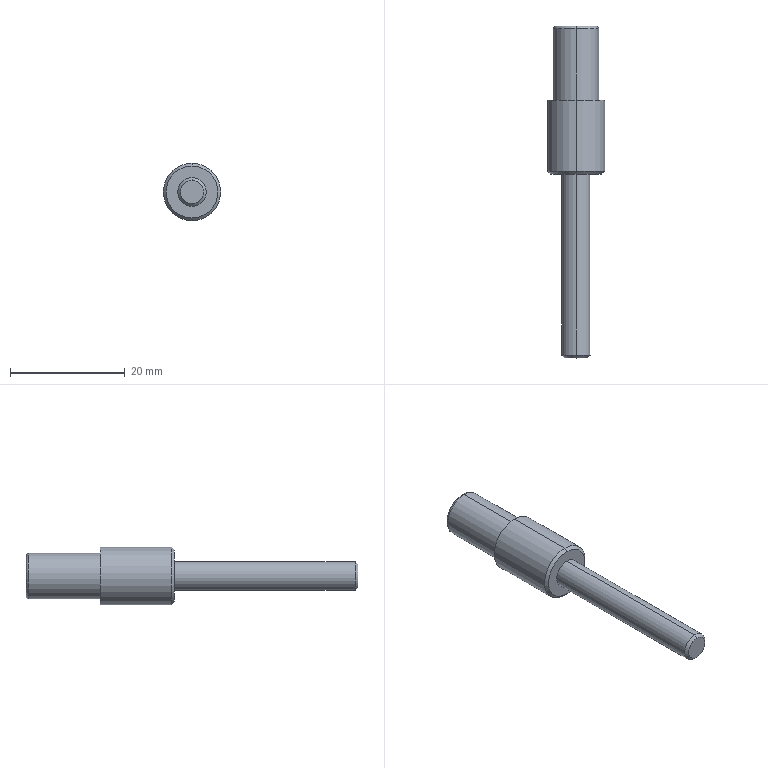Part | SolidWorks | features RefAxis 3, 3DProfileFeature 1, ICE 1, RevCut 1, Revolution 1 | 1 solid | 30 faces | box 10 x 57.8 x 10 mm | volume 2265 mm3 | plane 16 | cone 6 | cylinder 6 | torus 2 | commonest cylinder face diameters 5 x2 8 x2 10 x2
STEP:
#1=CARTESIAN_POINT('',(0.,22.934,0.));
#2=VERTEX_POINT('',#1);
#3=CARTESIAN_POINT('',(0.,23.8,1.5));
#4=VERTEX_POINT('',#3);
#5=CARTESIAN_POINT('',(0.,22.934,0.));
#6=DIRECTION('',(0.,0.5,0.866));
#7=VECTOR('',#6,1000.);
#8=LINE('',#5,#7);
#9=EDGE_CURVE('',#2,#4,#8,.T.);
#10=ORIENTED_EDGE('',*,*,#9,.F.);
#11=CARTESIAN_POINT('',(0.,23.8,-1.5));
#12=VERTEX_POINT('',#11);
#13=CARTESIAN_POINT('',(0.,22.934,0.));
#14=DIRECTION('',(0.,0.5,-0.866));
#15=VECTOR('',#14,1000.);
#16=LINE('',#13,#15);
#17=EDGE_CURVE('',#2,#12,#16,.T.);
#18=ORIENTED_EDGE('',*,*,#17,.T.);
#19=CARTESIAN_POINT('',(-0.75,23.8,-1.299));
#20=VERTEX_POINT('',#19);
#21=CARTESIAN_POINT('',(0.,23.8,0.));
#22=DIRECTION('',(0.,-1.,0.));
#23=DIRECTION('',(0.,0.,1.));
#24=AXIS2_PLACEMENT_3D('',#21,#22,#23);
#25=CIRCLE('',#24,1.5);
#26=EDGE_CURVE('',#20,#12,#25,.T.);
#27=ORIENTED_EDGE('',*,*,#26,.F.);
#28=CARTESIAN_POINT('',(-1.5,23.8,0.));
#29=VERTEX_POINT('',#28);
#30=CARTESIAN_POINT('',(0.,23.8,0.));
#31=DIRECTION('',(0.,-1.,0.));
#32=DIRECTION('',(0.,0.,1.));
#33=AXIS2_PLACEMENT_3D('',#30,#31,#32);
#34=CIRCLE('',#33,1.5);
#35=EDGE_CURVE('',#29,#20,#34,.T.);
#36=ORIENTED_EDGE('',*,*,#35,.F.);
#37=CARTESIAN_POINT('',(-0.75,23.8,1.299));
#38=VERTEX_POINT('',#37);
#39=CARTESIAN_POINT('',(0.,23.8,0.));
#40=DIRECTION('',(0.,-1.,0.));
#41=DIRECTION('',(0.,0.,1.));
#42=AXIS2_PLACEMENT_3D('',#39,#40,#41);
#43=CIRCLE('',#42,1.5);
#44=EDGE_CURVE('',#38,#29,#43,.T.);
#45=ORIENTED_EDGE('',*,*,#44,.F.);
#46=CARTESIAN_POINT('',(0.,23.8,0.));
#47=DIRECTION('',(0.,-1.,0.));
#48=DIRECTION('',(0.,0.,1.));
#49=AXIS2_PLACEMENT_3D('',#46,#47,#48);
#50=CIRCLE('',#49,1.5);
#51=EDGE_CURVE('',#4,#38,#50,.T.);
#52=ORIENTED_EDGE('',*,*,#51,.F.);
#53=EDGE_LOOP('',(#10,#18,#27,#36,#45,#52));
#54=FACE_OUTER_BOUND('',#53,.T.);
#55=CARTESIAN_POINT('',(0.,1022.934,0.));
#56=DIRECTION('',(0.,1.,0.));
#57=DIRECTION('',(0.,0.,1.));
#58=AXIS2_PLACEMENT_3D('',#55,#56,#57);
#59=CONICAL_SURFACE('',#58,1732.051,1.047);
#60=ADVANCED_FACE('',(#54),#59,.F.);
#61=CARTESIAN_POINT('',(0.,-32.,2.01));
#62=VERTEX_POINT('',#61);
#63=CARTESIAN_POINT('',(0.,-32.,-2.01));
#64=VERTEX_POINT('',#63);
#65=CARTESIAN_POINT('',(0.,-32.,0.));
#66=DIRECTION('',(0.,1.,0.));
#67=DIRECTION('',(0.,0.,1.));
#68=AXIS2_PLACEMENT_3D('',#65,#66,#67);
#69=CIRCLE('',#68,2.01);
#70=EDGE_CURVE('',#62,#64,#69,.T.);
#71=ORIENTED_EDGE('',*,*,#70,.T.);
#72=CARTESIAN_POINT('',(0.,-31.51,-2.5));
#73=VERTEX_POINT('',#72);
#74=CARTESIAN_POINT('',(0.,-32.,-2.01));
#75=DIRECTION('',(0.,0.7071,-0.7071));
#76=VECTOR('',#75,1000.);
#77=LINE('',#74,#76);
#78=EDGE_CURVE('',#64,#73,#77,.T.);
#79=ORIENTED_EDGE('',*,*,#78,.T.);
#80=CARTESIAN_POINT('',(0.,-31.51,2.5));
#81=VERTEX_POINT('',#80);
#82=CARTESIAN_POINT('',(0.,-31.51,0.));
#83=DIRECTION('',(0.,1.,0.));
#84=DIRECTION('',(0.,0.,1.));
#85=AXIS2_PLACEMENT_3D('',#82,#83,#84);
#86=CIRCLE('',#85,2.5);
#87=EDGE_CURVE('',#81,#73,#86,.T.);
#88=ORIENTED_EDGE('',*,*,#87,.F.);
#89=CARTESIAN_POINT('',(0.,-32.,2.01));
#90=DIRECTION('',(0.,0.7071,0.7071));
#91=VECTOR('',#90,1000.);
#92=LINE('',#89,#91);
#93=EDGE_CURVE('',#62,#81,#92,.T.);
#94=ORIENTED_EDGE('',*,*,#93,.F.);
#95=EDGE_LOOP('',(#71,#79,#88,#94));
#96=FACE_OUTER_BOUND('',#95,.T.);
#97=CARTESIAN_POINT('',(0.,-32.,0.));
#98=DIRECTION('',(0.,1.,0.));
#99=DIRECTION('',(0.,0.,1.));
#100=AXIS2_PLACEMENT_3D('',#97,#98,#99);
#101=CONICAL_SURFACE('',#100,2.01,0.7854);
#102=ADVANCED_FACE('',(#96),#101,.T.);
#103=ORIENTED_EDGE('',*,*,#87,.T.);
#104=CARTESIAN_POINT('',(0.,0.,-2.5));
#105=VERTEX_POINT('',#104);
#106=CARTESIAN_POINT('',(0.,-32.,-2.5));
#107=DIRECTION('',(0.,1.,0.));
#108=VECTOR('',#107,1000.);
#109=LINE('',#106,#108);
#110=EDGE_CURVE('',#73,#105,#109,.T.);
#111=ORIENTED_EDGE('',*,*,#110,.T.);
#112=CARTESIAN_POINT('',(0.,0.,2.5));
#113=VERTEX_POINT('',#112);
#114=CARTESIAN_POINT('',(0.,0.,0.));
#115=DIRECTION('',(0.,1.,0.));
#116=DIRECTION('',(0.,0.,1.));
#117=AXIS2_PLACEMENT_3D('',#114,#115,#116);
#118=CIRCLE('',#117,2.5);
#119=EDGE_CURVE('',#113,#105,#118,.T.);
#120=ORIENTED_EDGE('',*,*,#119,.F.);
#121=CARTESIAN_POINT('',(0.,-32.,2.5));
#122=DIRECTION('',(0.,1.,0.));
#123=VECTOR('',#122,1000.);
#124=LINE('',#121,#123);
#125=EDGE_CURVE('',#81,#113,#124,.T.);
#126=ORIENTED_EDGE('',*,*,#125,.F.);
#127=EDGE_LOOP('',(#103,#111,#120,#126));
#128=FACE_OUTER_BOUND('',#127,.T.);
#129=CARTESIAN_POINT('',(0.,-32.,0.));
#130=DIRECTION('',(0.,1.,0.));
#131=DIRECTION('',(0.,0.,1.));
#132=AXIS2_PLACEMENT_3D('',#129,#130,#131);
#133=CYLINDRICAL_SURFACE('',#132,2.5);
#134=ADVANCED_FACE('',(#128),#133,.T.);
#135=CARTESIAN_POINT('',(0.,0.,4.5));
#136=VERTEX_POINT('',#135);
#137=CARTESIAN_POINT('',(0.,0.,-4.5));
#138=VERTEX_POINT('',#137);
#139=CARTESIAN_POINT('',(0.,0.,0.));
#140=DIRECTION('',(0.,1.,0.));
#141=DIRECTION('',(0.,0.,1.));
#142=AXIS2_PLACEMENT_3D('',#139,#140,#141);
#143=CIRCLE('',#142,4.5);
#144=EDGE_CURVE('',#136,#138,#143,.T.);
#145=ORIENTED_EDGE('',*,*,#144,.T.);
#146=CARTESIAN_POINT('',(0.,0.5,-5.));
#147=VERTEX_POINT('',#146);
#148=CARTESIAN_POINT('',(0.,0.,-4.5));
#149=DIRECTION('',(0.,0.7071,-0.7071));
#150=VECTOR('',#149,1000.);
#151=LINE('',#148,#150);
#152=EDGE_CURVE('',#138,#147,#151,.T.);
#153=ORIENTED_EDGE('',*,*,#152,.T.);
#154=CARTESIAN_POINT('',(0.,0.5,5.));
#155=VERTEX_POINT('',#154);
#156=CARTESIAN_POINT('',(0.,0.5,0.));
#157=DIRECTION('',(0.,1.,0.));
#158=DIRECTION('',(0.,0.,1.));
#159=AXIS2_PLACEMENT_3D('',#156,#157,#158);
#160=CIRCLE('',#159,5.);
#161=EDGE_CURVE('',#155,#147,#160,.T.);
#162=ORIENTED_EDGE('',*,*,#161,.F.);
#163=CARTESIAN_POINT('',(0.,0.,4.5));
#164=DIRECTION('',(0.,0.7071,0.7071));
#165=VECTOR('',#164,1000.);
#166=LINE('',#163,#165);
#167=EDGE_CURVE('',#136,#155,#166,.T.);
#168=ORIENTED_EDGE('',*,*,#167,.F.);
#169=EDGE_LOOP('',(#145,#153,#162,#168));
#170=FACE_OUTER_BOUND('',#169,.T.);
#171=CARTESIAN_POINT('',(0.,0.,0.));
#172=DIRECTION('',(0.,1.,0.));
#173=DIRECTION('',(0.,0.,1.));
#174=AXIS2_PLACEMENT_3D('',#171,#172,#173);
#175=CONICAL_SURFACE('',#174,4.5,0.7854);
#176=ADVANCED_FACE('',(#170),#175,.T.);
#177=ORIENTED_EDGE('',*,*,#161,.T.);
#178=CARTESIAN_POINT('',(0.,12.9,-5.));
#179=VERTEX_POINT('',#178);
#180=CARTESIAN_POINT('',(0.,-32.,-5.));
#181=DIRECTION('',(0.,1.,0.));
#182=VECTOR('',#181,1000.);
#183=LINE('',#180,#182);
#184=EDGE_CURVE('',#147,#179,#183,.T.);
#185=ORIENTED_EDGE('',*,*,#184,.T.);
#186=CARTESIAN_POINT('',(0.,12.9,5.));
#187=VERTEX_POINT('',#186);
#188=CARTESIAN_POINT('',(0.,12.9,0.));
#189=DIRECTION('',(0.,1.,0.));
#190=DIRECTION('',(0.,0.,1.));
#191=AXIS2_PLACEMENT_3D('',#188,#189,#190);
#192=CIRCLE('',#191,5.);
#193=EDGE_CURVE('',#187,#179,#192,.T.);
#194=ORIENTED_EDGE('',*,*,#193,.F.);
#195=CARTESIAN_POINT('',(0.,-32.,5.));
#196=DIRECTION('',(0.,1.,0.));
#197=VECTOR('',#196,1000.);
#198=LINE('',#195,#197);
#199=EDGE_CURVE('',#155,#187,#198,.T.);
#200=ORIENTED_EDGE('',*,*,#199,.F.);
#201=EDGE_LOOP('',(#177,#185,#194,#200));
#202=FACE_OUTER_BOUND('',#201,.T.);
#203=CARTESIAN_POINT('',(0.,-32.,0.));
#204=DIRECTION('',(0.,1.,0.));
#205=DIRECTION('',(0.,0.,1.));
#206=AXIS2_PLACEMENT_3D('',#203,#204,#205);
#207=CYLINDRICAL_SURFACE('',#206,5.);
#208=ADVANCED_FACE('',(#202),#207,.T.);
#209=CARTESIAN_POINT('',(0.,12.9,4.));
#210=VERTEX_POINT('',#209);
#211=CARTESIAN_POINT('',(0.,12.9,-4.));
#212=VERTEX_POINT('',#211);
#213=CARTESIAN_POINT('',(0.,12.9,0.));
#214=DIRECTION('',(0.,1.,0.));
#215=DIRECTION('',(0.,0.,1.));
#216=AXIS2_PLACEMENT_3D('',#213,#214,#215);
#217=CIRCLE('',#216,4.);
#218=EDGE_CURVE('',#210,#212,#217,.T.);
#219=ORIENTED_EDGE('',*,*,#218,.T.);
#220=CARTESIAN_POINT('',(0.,25.3,-4.));
#221=VERTEX_POINT('',#220);
#222=CARTESIAN_POINT('',(0.,-32.,-4.));
#223=DIRECTION('',(0.,1.,0.));
#224=VECTOR('',#223,1000.);
#225=LINE('',#222,#224);
#226=EDGE_CURVE('',#212,#221,#225,.T.);
#227=ORIENTED_EDGE('',*,*,#226,.T.);
#228=CARTESIAN_POINT('',(0.,25.3,4.));
#229=VERTEX_POINT('',#228);
#230=CARTESIAN_POINT('',(0.,25.3,0.));
#231=DIRECTION('',(0.,1.,0.));
#232=DIRECTION('',(0.,0.,1.));
#233=AXIS2_PLACEMENT_3D('',#230,#231,#232);
#234=CIRCLE('',#233,4.);
#235=EDGE_CURVE('',#229,#221,#234,.T.);
#236=ORIENTED_EDGE('',*,*,#235,.F.);
#237=CARTESIAN_POINT('',(0.,-32.,4.));
#238=DIRECTION('',(0.,1.,0.));
#239=VECTOR('',#238,1000.);
#240=LINE('',#237,#239);
#241=EDGE_CURVE('',#210,#229,#240,.T.);
#242=ORIENTED_EDGE('',*,*,#241,.F.);
#243=EDGE_LOOP('',(#219,#227,#236,#242));
#244=FACE_OUTER_BOUND('',#243,.T.);
#245=CARTESIAN_POINT('',(0.,-32.,0.));
#246=DIRECTION('',(0.,1.,0.));
#247=DIRECTION('',(0.,0.,1.));
#248=AXIS2_PLACEMENT_3D('',#245,#246,#247);
#249=CYLINDRICAL_SURFACE('',#248,4.);
#250=ADVANCED_FACE('',(#244),#249,.T.);
#251=ORIENTED_EDGE('',*,*,#235,.T.);
#252=CARTESIAN_POINT('',(0.,25.8,-3.5));
#253=VERTEX_POINT('',#252);
#254=CARTESIAN_POINT('',(0.,25.3,-3.5));
#255=DIRECTION('',(1.,0.,0.));
#256=DIRECTION('',(0.,0.,-1.));
#257=AXIS2_PLACEMENT_3D('',#254,#255,#256);
#258=CIRCLE('',#257,0.5);
#259=EDGE_CURVE('',#221,#253,#258,.T.);
#260=ORIENTED_EDGE('',*,*,#259,.T.);
#261=CARTESIAN_POINT('',(0.,25.8,3.5));
#262=VERTEX_POINT('',#261);
#263=CARTESIAN_POINT('',(0.,25.8,0.));
#264=DIRECTION('',(0.,1.,0.));
#265=DIRECTION('',(0.,0.,1.));
#266=AXIS2_PLACEMENT_3D('',#263,#264,#265);
#267=CIRCLE('',#266,3.5);
#268=EDGE_CURVE('',#262,#253,#267,.T.);
#269=ORIENTED_EDGE('',*,*,#268,.F.);
#270=CARTESIAN_POINT('',(0.,25.3,3.5));
#271=DIRECTION('',(-1.,0.,0.));
#272=DIRECTION('',(0.,0.,1.));
#273=AXIS2_PLACEMENT_3D('',#270,#271,#272);
#274=CIRCLE('',#273,0.5);
#275=EDGE_CURVE('',#229,#262,#274,.T.);
#276=ORIENTED_EDGE('',*,*,#275,.F.);
#277=EDGE_LOOP('',(#251,#260,#269,#276));
#278=FACE_OUTER_BOUND('',#277,.T.);
#279=CARTESIAN_POINT('',(0.,25.3,0.));
#280=DIRECTION('',(0.,1.,0.));
#281=DIRECTION('',(0.,0.,1.));
#282=AXIS2_PLACEMENT_3D('',#279,#280,#281);
#283=TOROIDAL_SURFACE('',#282,3.5,0.5);
#284=ADVANCED_FACE('',(#278),#283,.T.);
#285=CARTESIAN_POINT('',(-1.5,23.8,0.866));
#286=VERTEX_POINT('',#285);
#287=CARTESIAN_POINT('',(-1.5,23.8,0.866));
#288=DIRECTION('',(0.866,0.,0.5));
#289=VECTOR('',#288,1000.);
#290=LINE('',#287,#289);
#291=EDGE_CURVE('',#286,#38,#290,.T.);
#292=ORIENTED_EDGE('',*,*,#291,.T.);
#293=ORIENTED_EDGE('',*,*,#44,.T.);
#294=CARTESIAN_POINT('',(-1.5,23.8,-0.866));
#295=DIRECTION('',(0.,0.,1.));
#296=VECTOR('',#295,1000.);
#297=LINE('',#294,#296);
#298=EDGE_CURVE('',#29,#286,#297,.T.);
#299=ORIENTED_EDGE('',*,*,#298,.T.);
#300=EDGE_LOOP('',(#292,#293,#299));
#301=FACE_OUTER_BOUND('',#300,.T.);
#302=CARTESIAN_POINT('',(-1.5,23.8,-0.866));
#303=DIRECTION('',(0.,1.,0.));
#304=DIRECTION('',(0.,0.,1.));
#305=AXIS2_PLACEMENT_3D('',#302,#303,#304);
#306=PLANE('',#305);
#307=ADVANCED_FACE('',(#301),#306,.T.);
#308=CARTESIAN_POINT('',(-1.5,23.8,-0.866));
#309=VERTEX_POINT('',#308);
#310=CARTESIAN_POINT('',(-1.5,23.8,-0.866));
#311=DIRECTION('',(0.,0.,1.));
#312=VECTOR('',#311,1000.);
#313=LINE('',#310,#312);
#314=EDGE_CURVE('',#309,#29,#313,.T.);
#315=ORIENTED_EDGE('',*,*,#314,.T.);
#316=ORIENTED_EDGE('',*,*,#35,.T.);
#317=CARTESIAN_POINT('',(0.,23.8,-1.732));
#318=DIRECTION('',(-0.866,0.,0.5));
#319=VECTOR('',#318,1000.);
#320=LINE('',#317,#319);
#321=EDGE_CURVE('',#20,#309,#320,.T.);
#322=ORIENTED_EDGE('',*,*,#321,.T.);
#323=EDGE_LOOP('',(#315,#316,#322));
#324=FACE_OUTER_BOUND('',#323,.T.);
#325=CARTESIAN_POINT('',(-1.5,23.8,-0.866));
#326=DIRECTION('',(0.,1.,0.));
#327=DIRECTION('',(0.,0.,1.));
#328=AXIS2_PLACEMENT_3D('',#325,#326,#327);
#329=PLANE('',#328);
#330=ADVANCED_FACE('',(#324),#329,.T.);
#331=CARTESIAN_POINT('',(0.,23.8,-1.732));
#332=VERTEX_POINT('',#331);
#333=CARTESIAN_POINT('',(0.,23.8,-1.732));
#334=DIRECTION('',(-0.866,0.,0.5));
#335=VECTOR('',#334,1000.);
#336=LINE('',#333,#335);
#337=EDGE_CURVE('',#332,#20,#336,.T.);
#338=ORIENTED_EDGE('',*,*,#337,.T.);
#339=ORIENTED_EDGE('',*,*,#26,.T.);
#340=CARTESIAN_POINT('',(0.75,23.8,-1.299));
#341=VERTEX_POINT('',#340);
#342=CARTESIAN_POINT('',(0.,23.8,0.));
#343=DIRECTION('',(0.,-1.,0.));
#344=DIRECTION('',(0.,0.,1.));
#345=AXIS2_PLACEMENT_3D('',#342,#343,#344);
#346=CIRCLE('',#345,1.5);
#347=EDGE_CURVE('',#12,#341,#346,.T.);
#348=ORIENTED_EDGE('',*,*,#347,.T.);
#349=CARTESIAN_POINT('',(1.5,23.8,-0.866));
#350=DIRECTION('',(-0.866,0.,-0.5));
#351=VECTOR('',#350,1000.);
#352=LINE('',#349,#351);
#353=EDGE_CURVE('',#341,#332,#352,.T.);
#354=ORIENTED_EDGE('',*,*,#353,.T.);
#355=EDGE_LOOP('',(#338,#339,#348,#354));
#356=FACE_OUTER_BOUND('',#355,.T.);
#357=CARTESIAN_POINT('',(-1.5,23.8,-0.866));
#358=DIRECTION('',(0.,1.,0.));
#359=DIRECTION('',(0.,0.,1.));
#360=AXIS2_PLACEMENT_3D('',#357,#358,#359);
#361=PLANE('',#360);
#362=ADVANCED_FACE('',(#356),#361,.T.);
#363=CARTESIAN_POINT('',(1.5,23.8,-0.866));
#364=VERTEX_POINT('',#363);
#365=CARTESIAN_POINT('',(1.5,23.8,-0.866));
#366=DIRECTION('',(-0.866,0.,-0.5));
#367=VECTOR('',#366,1000.);
#368=LINE('',#365,#367);
#369=EDGE_CURVE('',#364,#341,#368,.T.);
#370=ORIENTED_EDGE('',*,*,#369,.T.);
#371=CARTESIAN_POINT('',(1.5,23.8,0.));
#372=VERTEX_POINT('',#371);
#373=CARTESIAN_POINT('',(0.,23.8,0.));
#374=DIRECTION('',(0.,-1.,0.));
#375=DIRECTION('',(0.,0.,1.));
#376=AXIS2_PLACEMENT_3D('',#373,#374,#375);
#377=CIRCLE('',#376,1.5);
#378=EDGE_CURVE('',#341,#372,#377,.T.);
#379=ORIENTED_EDGE('',*,*,#378,.T.);
#380=CARTESIAN_POINT('',(1.5,23.8,0.866));
#381=DIRECTION('',(0.,0.,-1.));
#382=VECTOR('',#381,1000.);
#383=LINE('',#380,#382);
#384=EDGE_CURVE('',#372,#364,#383,.T.);
#385=ORIENTED_EDGE('',*,*,#384,.T.);
#386=EDGE_LOOP('',(#370,#379,#385));
#387=FACE_OUTER_BOUND('',#386,.T.);
#388=CARTESIAN_POINT('',(-1.5,23.8,-0.866));
#389=DIRECTION('',(0.,1.,0.));
#390=DIRECTION('',(0.,0.,1.));
#391=AXIS2_PLACEMENT_3D('',#388,#389,#390);
#392=PLANE('',#391);
#393=ADVANCED_FACE('',(#387),#392,.T.);
#394=CARTESIAN_POINT('',(1.5,23.8,0.866));
#395=VERTEX_POINT('',#394);
#396=CARTESIAN_POINT('',(1.5,23.8,0.866));
#397=DIRECTION('',(0.,0.,-1.));
#398=VECTOR('',#397,1000.);
#399=LINE('',#396,#398);
#400=EDGE_CURVE('',#395,#372,#399,.T.);
#401=ORIENTED_EDGE('',*,*,#400,.T.);
#402=CARTESIAN_POINT('',(0.75,23.8,1.299));
#403=VERTEX_POINT('',#402);
#404=CARTESIAN_POINT('',(0.,23.8,0.));
#405=DIRECTION('',(0.,1.,0.));
#406=DIRECTION('',(0.,0.,1.));
#407=AXIS2_PLACEMENT_3D('',#404,#405,#406);
#408=CIRCLE('',#407,1.5);
#409=EDGE_CURVE('',#403,#372,#408,.T.);
#410=ORIENTED_EDGE('',*,*,#409,.F.);
#411=CARTESIAN_POINT('',(0.,23.8,1.732));
#412=DIRECTION('',(0.866,0.,-0.5));
#413=VECTOR('',#412,1000.);
#414=LINE('',#411,#413);
#415=EDGE_CURVE('',#403,#395,#414,.T.);
#416=ORIENTED_EDGE('',*,*,#415,.T.);
#417=EDGE_LOOP('',(#401,#410,#416));
#418=FACE_OUTER_BOUND('',#417,.T.);
#419=CARTESIAN_POINT('',(-1.5,23.8,-0.866));
#420=DIRECTION('',(0.,1.,0.));
#421=DIRECTION('',(0.,0.,1.));
#422=AXIS2_PLACEMENT_3D('',#419,#420,#421);
#423=PLANE('',#422);
#424=ADVANCED_FACE('',(#418),#423,.T.);
#425=CARTESIAN_POINT('',(0.,23.8,1.732));
#426=VERTEX_POINT('',#425);
#427=CARTESIAN_POINT('',(0.,23.8,1.732));
#428=DIRECTION('',(0.866,0.,-0.5));
#429=VECTOR('',#428,1000.);
#430=LINE('',#427,#429);
#431=EDGE_CURVE('',#426,#403,#430,.T.);
#432=ORIENTED_EDGE('',*,*,#431,.T.);
#433=CARTESIAN_POINT('',(0.,23.8,0.));
#434=DIRECTION('',(0.,-1.,0.));
#435=DIRECTION('',(0.,0.,1.));
#436=AXIS2_PLACEMENT_3D('',#433,#434,#435);
#437=CIRCLE('',#436,1.5);
#438=EDGE_CURVE('',#403,#4,#437,.T.);
#439=ORIENTED_EDGE('',*,*,#438,.T.);
#440=ORIENTED_EDGE('',*,*,#51,.T.);
#441=CARTESIAN_POINT('',(-1.5,23.8,0.866));
#442=DIRECTION('',(0.866,0.,0.5));
#443=VECTOR('',#442,1000.);
#444=LINE('',#441,#443);
#445=EDGE_CURVE('',#38,#426,#444,.T.);
#446=ORIENTED_EDGE('',*,*,#445,.T.);
#447=EDGE_LOOP('',(#432,#439,#440,#446));
#448=FACE_OUTER_BOUND('',#447,.T.);
#449=CARTESIAN_POINT('',(-1.5,23.8,-0.866));
#450=DIRECTION('',(0.,1.,0.));
#451=DIRECTION('',(0.,0.,1.));
#452=AXIS2_PLACEMENT_3D('',#449,#450,#451);
#453=PLANE('',#452);
#454=ADVANCED_FACE('',(#448),#453,.T.);
#455=CARTESIAN_POINT('',(-1.5,25.8,0.866));
#456=VERTEX_POINT('',#455);
#457=CARTESIAN_POINT('',(-1.5,25.8,-0.866));
#458=VERTEX_POINT('',#457);
#459=CARTESIAN_POINT('',(-1.5,25.8,0.));
#460=DIRECTION('',(0.,0.,-1.));
#461=VECTOR('',#460,1000.);
#462=LINE('',#459,#461);
#463=EDGE_CURVE('',#456,#458,#462,.T.);
#464=ORIENTED_EDGE('',*,*,#463,.T.);
#465=CARTESIAN_POINT('',(0.,25.8,-1.732));
#466=VERTEX_POINT('',#465);
#467=CARTESIAN_POINT('',(-0.75,25.8,-1.299));
#468=DIRECTION('',(0.866,0.,-0.5));
#469=VECTOR('',#468,1000.);
#470=LINE('',#467,#469);
#471=EDGE_CURVE('',#458,#466,#470,.T.);
#472=ORIENTED_EDGE('',*,*,#471,.T.);
#473=CARTESIAN_POINT('',(1.5,25.8,-0.866));
#474=VERTEX_POINT('',#473);
#475=CARTESIAN_POINT('',(0.75,25.8,-1.299));
#476=DIRECTION('',(0.866,0.,0.5));
#477=VECTOR('',#476,1000.);
#478=LINE('',#475,#477);
#479=EDGE_CURVE('',#466,#474,#478,.T.);
#480=ORIENTED_EDGE('',*,*,#479,.T.);
#481=CARTESIAN_POINT('',(1.5,25.8,0.866));
#482=VERTEX_POINT('',#481);
#483=CARTESIAN_POINT('',(1.5,25.8,0.));
#484=DIRECTION('',(0.,0.,1.));
#485=VECTOR('',#484,1000.);
#486=LINE('',#483,#485);
#487=EDGE_CURVE('',#474,#482,#486,.T.);
#488=ORIENTED_EDGE('',*,*,#487,.T.);
#489=CARTESIAN_POINT('',(0.,25.8,1.732));
#490=VERTEX_POINT('',#489);
#491=CARTESIAN_POINT('',(0.75,25.8,1.299));
#492=DIRECTION('',(-0.866,0.,0.5));
#493=VECTOR('',#492,1000.);
#494=LINE('',#491,#493);
#495=EDGE_CURVE('',#482,#490,#494,.T.);
#496=ORIENTED_EDGE('',*,*,#495,.T.);
#497=CARTESIAN_POINT('',(-0.75,25.8,1.299));
#498=DIRECTION('',(-0.866,0.,-0.5));
#499=VECTOR('',#498,1000.);
#500=LINE('',#497,#499);
#501=EDGE_CURVE('',#490,#456,#500,.T.);
#502=ORIENTED_EDGE('',*,*,#501,.T.);
#503=EDGE_LOOP('',(#464,#472,#480,#488,#496,#502));
#504=FACE_BOUND('',#503,.T.);
#505=ORIENTED_EDGE('',*,*,#268,.T.);
#506=CARTESIAN_POINT('',(0.,25.8,0.));
#507=DIRECTION('',(0.,1.,0.));
#508=DIRECTION('',(0.,0.,1.));
#509=AXIS2_PLACEMENT_3D('',#506,#507,#508);
#510=CIRCLE('',#509,3.5);
#511=EDGE_CURVE('',#253,#262,#510,.T.);
#512=ORIENTED_EDGE('',*,*,#511,.T.);
#513=EDGE_LOOP('',(#505,#512));
#514=FACE_OUTER_BOUND('',#513,.T.);
#515=CARTESIAN_POINT('',(0.,25.8,0.));
#516=DIRECTION('',(0.,-1.,0.));
#517=DIRECTION('',(0.,0.,-1.));
#518=AXIS2_PLACEMENT_3D('',#515,#516,#517);
#519=PLANE('',#518);
#520=ADVANCED_FACE('',(#504,#514),#519,.F.);
#521=ORIENTED_EDGE('',*,*,#259,.F.);
#522=CARTESIAN_POINT('',(0.,25.3,0.));
#523=DIRECTION('',(0.,1.,0.));
#524=DIRECTION('',(0.,0.,1.));
#525=AXIS2_PLACEMENT_3D('',#522,#523,#524);
#526=CIRCLE('',#525,4.);
#527=EDGE_CURVE('',#221,#229,#526,.T.);
#528=ORIENTED_EDGE('',*,*,#527,.T.);
#529=ORIENTED_EDGE('',*,*,#275,.T.);
#530=ORIENTED_EDGE('',*,*,#511,.F.);
#531=EDGE_LOOP('',(#521,#528,#529,#530));
#532=FACE_OUTER_BOUND('',#531,.T.);
#533=CARTESIAN_POINT('',(0.,25.3,0.));
#534=DIRECTION('',(0.,1.,0.));
#535=DIRECTION('',(0.,0.,1.));
#536=AXIS2_PLACEMENT_3D('',#533,#534,#535);
#537=TOROIDAL_SURFACE('',#536,3.5,0.5);
#538=ADVANCED_FACE('',(#532),#537,.T.);
#539=ORIENTED_EDGE('',*,*,#226,.F.);
#540=CARTESIAN_POINT('',(0.,12.9,0.));
#541=DIRECTION('',(0.,1.,0.));
#542=DIRECTION('',(0.,0.,1.));
#543=AXIS2_PLACEMENT_3D('',#540,#541,#542);
#544=CIRCLE('',#543,4.);
#545=EDGE_CURVE('',#212,#210,#544,.T.);
#546=ORIENTED_EDGE('',*,*,#545,.T.);
#547=ORIENTED_EDGE('',*,*,#241,.T.);
#548=ORIENTED_EDGE('',*,*,#527,.F.);
#549=EDGE_LOOP('',(#539,#546,#547,#548));
#550=FACE_OUTER_BOUND('',#549,.T.);
#551=CARTESIAN_POINT('',(0.,-32.,0.));
#552=DIRECTION('',(0.,1.,0.));
#553=DIRECTION('',(0.,0.,1.));
#554=AXIS2_PLACEMENT_3D('',#551,#552,#553);
#555=CYLINDRICAL_SURFACE('',#554,4.);
#556=ADVANCED_FACE('',(#550),#555,.T.);
#557=ORIENTED_EDGE('',*,*,#218,.F.);
#558=ORIENTED_EDGE('',*,*,#545,.F.);
#559=EDGE_LOOP('',(#557,#558));
#560=FACE_BOUND('',#559,.T.);
#561=ORIENTED_EDGE('',*,*,#193,.T.);
#562=CARTESIAN_POINT('',(0.,12.9,0.));
#563=DIRECTION('',(0.,1.,0.));
#564=DIRECTION('',(0.,0.,1.));
#565=AXIS2_PLACEMENT_3D('',#562,#563,#564);
#566=CIRCLE('',#565,5.);
#567=EDGE_CURVE('',#179,#187,#566,.T.);
#568=ORIENTED_EDGE('',*,*,#567,.T.);
#569=EDGE_LOOP('',(#561,#568));
#570=FACE_OUTER_BOUND('',#569,.T.);
#571=CARTESIAN_POINT('',(4.,12.9,0.));
#572=DIRECTION('',(0.,-1.,0.));
#573=DIRECTION('',(0.,0.,-1.));
#574=AXIS2_PLACEMENT_3D('',#571,#572,#573);
#575=PLANE('',#574);
#576=ADVANCED_FACE('',(#560,#570),#575,.F.);
#577=ORIENTED_EDGE('',*,*,#184,.F.);
#578=CARTESIAN_POINT('',(0.,0.5,0.));
#579=DIRECTION('',(0.,1.,0.));
#580=DIRECTION('',(0.,0.,1.));
#581=AXIS2_PLACEMENT_3D('',#578,#579,#580);
#582=CIRCLE('',#581,5.);
#583=EDGE_CURVE('',#147,#155,#582,.T.);
#584=ORIENTED_EDGE('',*,*,#583,.T.);
#585=ORIENTED_EDGE('',*,*,#199,.T.);
#586=ORIENTED_EDGE('',*,*,#567,.F.);
#587=EDGE_LOOP('',(#577,#584,#585,#586));
#588=FACE_OUTER_BOUND('',#587,.T.);
#589=CARTESIAN_POINT('',(0.,-32.,0.));
#590=DIRECTION('',(0.,1.,0.));
#591=DIRECTION('',(0.,0.,1.));
#592=AXIS2_PLACEMENT_3D('',#589,#590,#591);
#593=CYLINDRICAL_SURFACE('',#592,5.);
#594=ADVANCED_FACE('',(#588),#593,.T.);
#595=ORIENTED_EDGE('',*,*,#152,.F.);
#596=CARTESIAN_POINT('',(0.,0.,0.));
#597=DIRECTION('',(0.,1.,0.));
#598=DIRECTION('',(0.,0.,1.));
#599=AXIS2_PLACEMENT_3D('',#596,#597,#598);
#600=CIRCLE('',#599,4.5);
#601=EDGE_CURVE('',#138,#136,#600,.T.);
#602=ORIENTED_EDGE('',*,*,#601,.T.);
#603=ORIENTED_EDGE('',*,*,#167,.T.);
#604=ORIENTED_EDGE('',*,*,#583,.F.);
#605=EDGE_LOOP('',(#595,#602,#603,#604));
#606=FACE_OUTER_BOUND('',#605,.T.);
#607=CARTESIAN_POINT('',(0.,0.,0.));
#608=DIRECTION('',(0.,1.,0.));
#609=DIRECTION('',(0.,0.,1.));
#610=AXIS2_PLACEMENT_3D('',#607,#608,#609);
#611=CONICAL_SURFACE('',#610,4.5,0.7854);
#612=ADVANCED_FACE('',(#606),#611,.T.);
#613=ORIENTED_EDGE('',*,*,#144,.F.);
#614=ORIENTED_EDGE('',*,*,#601,.F.);
#615=EDGE_LOOP('',(#613,#614));
#616=FACE_OUTER_BOUND('',#615,.T.);
#617=ORIENTED_EDGE('',*,*,#119,.T.);
#618=CARTESIAN_POINT('',(0.,0.,0.));
#619=DIRECTION('',(0.,1.,0.));
#620=DIRECTION('',(0.,0.,1.));
#621=AXIS2_PLACEMENT_3D('',#618,#619,#620);
#622=CIRCLE('',#621,2.5);
#623=EDGE_CURVE('',#105,#113,#622,.T.);
#624=ORIENTED_EDGE('',*,*,#623,.T.);
#625=EDGE_LOOP('',(#617,#624));
#626=FACE_BOUND('',#625,.T.);
#627=CARTESIAN_POINT('',(4.5,0.,0.));
#628=DIRECTION('',(0.,1.,0.));
#629=DIRECTION('',(0.,0.,1.));
#630=AXIS2_PLACEMENT_3D('',#627,#628,#629);
#631=PLANE('',#630);
#632=ADVANCED_FACE('',(#616,#626),#631,.F.);
#633=ORIENTED_EDGE('',*,*,#110,.F.);
#634=CARTESIAN_POINT('',(0.,-31.51,0.));
#635=DIRECTION('',(0.,1.,0.));
#636=DIRECTION('',(0.,0.,1.));
#637=AXIS2_PLACEMENT_3D('',#634,#635,#636);
#638=CIRCLE('',#637,2.5);
#639=EDGE_CURVE('',#73,#81,#638,.T.);
#640=ORIENTED_EDGE('',*,*,#639,.T.);
#641=ORIENTED_EDGE('',*,*,#125,.T.);
#642=ORIENTED_EDGE('',*,*,#623,.F.);
#643=EDGE_LOOP('',(#633,#640,#641,#642));
#644=FACE_OUTER_BOUND('',#643,.T.);
#645=CARTESIAN_POINT('',(0.,-32.,0.));
#646=DIRECTION('',(0.,1.,0.));
#647=DIRECTION('',(0.,0.,1.));
#648=AXIS2_PLACEMENT_3D('',#645,#646,#647);
#649=CYLINDRICAL_SURFACE('',#648,2.5);
#650=ADVANCED_FACE('',(#644),#649,.T.);
#651=ORIENTED_EDGE('',*,*,#78,.F.);
#652=CARTESIAN_POINT('',(0.,-32.,0.));
#653=DIRECTION('',(0.,1.,0.));
#654=DIRECTION('',(0.,0.,1.));
#655=AXIS2_PLACEMENT_3D('',#652,#653,#654);
#656=CIRCLE('',#655,2.01);
#657=EDGE_CURVE('',#64,#62,#656,.T.);
#658=ORIENTED_EDGE('',*,*,#657,.T.);
#659=ORIENTED_EDGE('',*,*,#93,.T.);
#660=ORIENTED_EDGE('',*,*,#639,.F.);
#661=EDGE_LOOP('',(#651,#658,#659,#660));
#662=FACE_OUTER_BOUND('',#661,.T.);
#663=CARTESIAN_POINT('',(0.,-32.,0.));
#664=DIRECTION('',(0.,1.,0.));
#665=DIRECTION('',(0.,0.,1.));
#666=AXIS2_PLACEMENT_3D('',#663,#664,#665);
#667=CONICAL_SURFACE('',#666,2.01,0.7854);
#668=ADVANCED_FACE('',(#662),#667,.T.);
#669=ORIENTED_EDGE('',*,*,#70,.F.);
#670=ORIENTED_EDGE('',*,*,#657,.F.);
#671=EDGE_LOOP('',(#669,#670));
#672=FACE_OUTER_BOUND('',#671,.T.);
#673=CARTESIAN_POINT('',(2.01,-32.,0.));
#674=DIRECTION('',(0.,1.,0.));
#675=DIRECTION('',(0.,0.,1.));
#676=AXIS2_PLACEMENT_3D('',#673,#674,#675);
#677=PLANE('',#676);
#678=ADVANCED_FACE('',(#672),#677,.F.);
#679=CARTESIAN_POINT('',(0.,23.8,-1.732));
#680=DIRECTION('',(0.,1.,0.));
#681=VECTOR('',#680,1000.);
#682=LINE('',#679,#681);
#683=EDGE_CURVE('',#332,#466,#682,.T.);
#684=ORIENTED_EDGE('',*,*,#683,.T.);
#685=ORIENTED_EDGE('',*,*,#471,.F.);
#686=CARTESIAN_POINT('',(-1.5,23.8,-0.866));
#687=DIRECTION('',(0.,1.,0.));
#688=VECTOR('',#687,1000.);
#689=LINE('',#686,#688);
#690=EDGE_CURVE('',#309,#458,#689,.T.);
#691=ORIENTED_EDGE('',*,*,#690,.F.);
#692=ORIENTED_EDGE('',*,*,#321,.F.);
#693=ORIENTED_EDGE('',*,*,#337,.F.);
#694=EDGE_LOOP('',(#684,#685,#691,#692,#693));
#695=FACE_OUTER_BOUND('',#694,.T.);
#696=CARTESIAN_POINT('',(0.,23.8,-1.732));
#697=DIRECTION('',(-0.5,0.,-0.866));
#698=DIRECTION('',(-0.866,0.,0.5));
#699=AXIS2_PLACEMENT_3D('',#696,#697,#698);
#700=PLANE('',#699);
#701=ADVANCED_FACE('',(#695),#700,.F.);
#702=CARTESIAN_POINT('',(1.5,23.8,-0.866));
#703=DIRECTION('',(0.,1.,0.));
#704=VECTOR('',#703,1000.);
#705=LINE('',#702,#704);
#706=EDGE_CURVE('',#364,#474,#705,.T.);
#707=ORIENTED_EDGE('',*,*,#706,.T.);
#708=ORIENTED_EDGE('',*,*,#479,.F.);
#709=ORIENTED_EDGE('',*,*,#683,.F.);
#710=ORIENTED_EDGE('',*,*,#353,.F.);
#711=ORIENTED_EDGE('',*,*,#369,.F.);
#712=EDGE_LOOP('',(#707,#708,#709,#710,#711));
#713=FACE_OUTER_BOUND('',#712,.T.);
#714=CARTESIAN_POINT('',(1.5,23.8,-0.866));
#715=DIRECTION('',(0.5,0.,-0.866));
#716=DIRECTION('',(-0.866,0.,-0.5));
#717=AXIS2_PLACEMENT_3D('',#714,#715,#716);
#718=PLANE('',#717);
#719=ADVANCED_FACE('',(#713),#718,.F.);
#720=CARTESIAN_POINT('',(1.5,23.8,0.866));
#721=DIRECTION('',(0.,1.,0.));
#722=VECTOR('',#721,1000.);
#723=LINE('',#720,#722);
#724=EDGE_CURVE('',#395,#482,#723,.T.);
#725=ORIENTED_EDGE('',*,*,#724,.T.);
#726=ORIENTED_EDGE('',*,*,#487,.F.);
#727=ORIENTED_EDGE('',*,*,#706,.F.);
#728=ORIENTED_EDGE('',*,*,#384,.F.);
#729=ORIENTED_EDGE('',*,*,#400,.F.);
#730=EDGE_LOOP('',(#725,#726,#727,#728,#729));
#731=FACE_OUTER_BOUND('',#730,.T.);
#732=CARTESIAN_POINT('',(1.5,23.8,0.866));
#733=DIRECTION('',(1.,0.,0.));
#734=DIRECTION('',(0.,0.,-1.));
#735=AXIS2_PLACEMENT_3D('',#732,#733,#734);
#736=PLANE('',#735);
#737=ADVANCED_FACE('',(#731),#736,.F.);
#738=CARTESIAN_POINT('',(0.,23.8,1.732));
#739=DIRECTION('',(0.,1.,0.));
#740=VECTOR('',#739,1000.);
#741=LINE('',#738,#740);
#742=EDGE_CURVE('',#426,#490,#741,.T.);
#743=ORIENTED_EDGE('',*,*,#742,.T.);
#744=ORIENTED_EDGE('',*,*,#495,.F.);
#745=ORIENTED_EDGE('',*,*,#724,.F.);
#746=ORIENTED_EDGE('',*,*,#415,.F.);
#747=ORIENTED_EDGE('',*,*,#431,.F.);
#748=EDGE_LOOP('',(#743,#744,#745,#746,#747));
#749=FACE_OUTER_BOUND('',#748,.T.);
#750=CARTESIAN_POINT('',(0.,23.8,1.732));
#751=DIRECTION('',(0.5,0.,0.866));
#752=DIRECTION('',(0.866,0.,-0.5));
#753=AXIS2_PLACEMENT_3D('',#750,#751,#752);
#754=PLANE('',#753);
#755=ADVANCED_FACE('',(#749),#754,.F.);
#756=CARTESIAN_POINT('',(-1.5,23.8,0.866));
#757=DIRECTION('',(0.,1.,0.));
#758=VECTOR('',#757,1000.);
#759=LINE('',#756,#758);
#760=EDGE_CURVE('',#286,#456,#759,.T.);
#761=ORIENTED_EDGE('',*,*,#760,.T.);
#762=ORIENTED_EDGE('',*,*,#501,.F.);
#763=ORIENTED_EDGE('',*,*,#742,.F.);
#764=ORIENTED_EDGE('',*,*,#445,.F.);
#765=ORIENTED_EDGE('',*,*,#291,.F.);
#766=EDGE_LOOP('',(#761,#762,#763,#764,#765));
#767=FACE_OUTER_BOUND('',#766,.T.);
#768=CARTESIAN_POINT('',(-1.5,23.8,0.866));
#769=DIRECTION('',(-0.5,0.,0.866));
#770=DIRECTION('',(0.866,0.,0.5));
#771=AXIS2_PLACEMENT_3D('',#768,#769,#770);
#772=PLANE('',#771);
#773=ADVANCED_FACE('',(#767),#772,.F.);
#774=ORIENTED_EDGE('',*,*,#690,.T.);
#775=ORIENTED_EDGE('',*,*,#463,.F.);
#776=ORIENTED_EDGE('',*,*,#760,.F.);
#777=ORIENTED_EDGE('',*,*,#298,.F.);
#778=ORIENTED_EDGE('',*,*,#314,.F.);
#779=EDGE_LOOP('',(#774,#775,#776,#777,#778));
#780=FACE_OUTER_BOUND('',#779,.T.);
#781=CARTESIAN_POINT('',(-1.5,23.8,-0.866));
#782=DIRECTION('',(-1.,0.,0.));
#783=DIRECTION('',(0.,0.,1.));
#784=AXIS2_PLACEMENT_3D('',#781,#782,#783);
#785=PLANE('',#784);
#786=ADVANCED_FACE('',(#780),#785,.F.);
#787=ORIENTED_EDGE('',*,*,#17,.F.);
#788=ORIENTED_EDGE('',*,*,#9,.T.);
#789=ORIENTED_EDGE('',*,*,#438,.F.);
#790=ORIENTED_EDGE('',*,*,#409,.T.);
#791=ORIENTED_EDGE('',*,*,#378,.F.);
#792=ORIENTED_EDGE('',*,*,#347,.F.);
#793=EDGE_LOOP('',(#787,#788,#789,#790,#791,#792));
#794=FACE_OUTER_BOUND('',#793,.T.);
#795=CARTESIAN_POINT('',(0.,1022.934,0.));
#796=DIRECTION('',(0.,1.,0.));
#797=DIRECTION('',(0.,0.,1.));
#798=AXIS2_PLACEMENT_3D('',#795,#796,#797);
#799=CONICAL_SURFACE('',#798,1732.051,1.047);
#800=ADVANCED_FACE('',(#794),#799,.F.);
#801=CLOSED_SHELL('',(#60,#102,#134,#176,#208,#250,#284,#307,#330,#362,#393,#424,#454,#520,#538,#556,#576,#594,#612,#632,#650,#668,#678,#701,#719,#737,#755,#773,#786,#800));
#802=MANIFOLD_SOLID_BREP('',#801);
#803=CARTESIAN_POINT('',(0.,0.,0.));
#804=DIRECTION('',(0.,0.,1.));
#805=DIRECTION('',(1.,0.,0.));
#806=AXIS2_PLACEMENT_3D('',#803,#804,#805);
#807=(LENGTH_UNIT()NAMED_UNIT(*)SI_UNIT(.MILLI.,.METRE.));
#808=UNCERTAINTY_MEASURE_WITH_UNIT(LENGTH_MEASURE(0.00001),#807,'','');
#809=(NAMED_UNIT(*)PLANE_ANGLE_UNIT()SI_UNIT($,.RADIAN.));
#810=(NAMED_UNIT(*)SI_UNIT($,.STERADIAN.)SOLID_ANGLE_UNIT());
#811=(GEOMETRIC_REPRESENTATION_CONTEXT(3)GLOBAL_UNCERTAINTY_ASSIGNED_CONTEXT((#808))GLOBAL_UNIT_ASSIGNED_CONTEXT((#807,#809,#810))REPRESENTATION_CONTEXT('',''));
#812=ADVANCED_BREP_SHAPE_REPRESENTATION('',(#802,#806),#811);